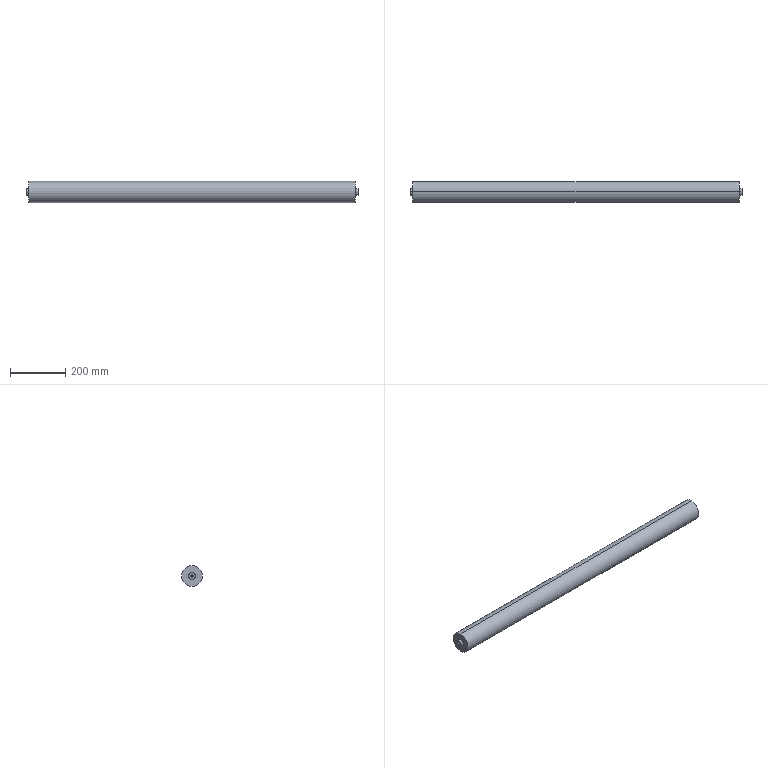Part | STEP file | φ76-1200 | 1 solid | 18 faces | box 1200 x 76 x 76 mm | volume 5359963 mm3 | cylinder 10 | cone 4 | plane 4 | commonest cylinder face diameters 8.5 x4 25 x4 76 x2
STEP:
#1=CARTESIAN_POINT('',(0.,0.,0.));
#2=DIRECTION('',(0.,0.,1.));
#3=DIRECTION('',(1.,0.,0.));
#4=AXIS2_PLACEMENT_3D('',#1,#2,#3);
#5=CARTESIAN_POINT('',(1175.5,0.,-4.25));
#6=VERTEX_POINT('',#5);
#7=CARTESIAN_POINT('',(1200.,0.,-4.25));
#8=VERTEX_POINT('',#7);
#9=CARTESIAN_POINT('',(1200.,0.,-4.25));
#10=DIRECTION('',(1.,0.,0.));
#11=VECTOR('',#10,1.);
#12=LINE('',#9,#11);
#13=CARTESIAN_POINT('',(1200.,0.,0.));
#14=DIRECTION('',(1.,0.,0.));
#15=DIRECTION('',(0.,0.,-1.));
#16=AXIS2_PLACEMENT_3D('',#13,#14,#15);
#17=CYLINDRICAL_SURFACE('',#16,4.25);
#18=CARTESIAN_POINT('',(6.283,0.));
#19=DIRECTION('',(0.,1.));
#20=VECTOR('',#19,1.);
#21=LINE('',#18,#20);
#22=(GEOMETRIC_REPRESENTATION_CONTEXT(2)PARAMETRIC_REPRESENTATION_CONTEXT()REPRESENTATION_CONTEXT('',''));
#23=DEFINITIONAL_REPRESENTATION('',(#21),#22);
#24=PCURVE('',#17,#23);
#25=CARTESIAN_POINT('',(1200.,0.,0.));
#26=DIRECTION('',(1.,0.,0.));
#27=DIRECTION('',(0.,0.,-1.));
#28=AXIS2_PLACEMENT_3D('',#25,#26,#27);
#29=CYLINDRICAL_SURFACE('',#28,4.25);
#30=CARTESIAN_POINT('',(0.,0.));
#31=DIRECTION('',(0.,1.));
#32=VECTOR('',#31,1.);
#33=LINE('',#30,#32);
#34=(GEOMETRIC_REPRESENTATION_CONTEXT(2)PARAMETRIC_REPRESENTATION_CONTEXT()REPRESENTATION_CONTEXT('',''));
#35=DEFINITIONAL_REPRESENTATION('',(#33),#34);
#36=PCURVE('',#29,#35);
#37=SURFACE_CURVE('',#12,(#24,#36),.PCURVE_S1.);
#38=EDGE_CURVE('',#6,#8,#37,.T.);
#39=ORIENTED_EDGE('',*,*,#38,.T.);
#40=CARTESIAN_POINT('',(1200.,0.,4.25));
#41=VERTEX_POINT('',#40);
#42=CARTESIAN_POINT('',(1200.,0.,0.));
#43=DIRECTION('',(1.,0.,0.));
#44=DIRECTION('',(0.,0.,-1.));
#45=AXIS2_PLACEMENT_3D('',#42,#43,#44);
#46=CIRCLE('',#45,4.25);
#47=CARTESIAN_POINT('',(0.,0.));
#48=DIRECTION('',(1.,0.));
#49=VECTOR('',#48,1.);
#50=LINE('',#47,#49);
#51=(GEOMETRIC_REPRESENTATION_CONTEXT(2)PARAMETRIC_REPRESENTATION_CONTEXT()REPRESENTATION_CONTEXT('',''));
#52=DEFINITIONAL_REPRESENTATION('',(#50),#51);
#53=PCURVE('',#17,#52);
#54=CARTESIAN_POINT('',(1200.,0.,0.));
#55=DIRECTION('',(-1.,0.,0.));
#56=DIRECTION('',(0.,0.,1.));
#57=AXIS2_PLACEMENT_3D('',#54,#55,#56);
#58=PLANE('',#57);
#59=CARTESIAN_POINT('',(-4.25,0.));
#60=CARTESIAN_POINT('',(-4.25,7.361));
#61=CARTESIAN_POINT('',(2.125,3.681));
#62=CARTESIAN_POINT('',(8.5,0.));
#63=CARTESIAN_POINT('',(2.125,-3.681));
#64=CARTESIAN_POINT('',(-4.25,-7.361));
#65=CARTESIAN_POINT('',(-4.25,0.));
#66=(BOUNDED_CURVE()B_SPLINE_CURVE(2,(#59,#60,#61,#62,#63,#64,#65),.UNSPECIFIED.,.T.,.F.)B_SPLINE_CURVE_WITH_KNOTS((1,2,2,2,2,1),(-2.094,0.,2.094,4.189,6.283,8.378),.UNSPECIFIED.)CURVE()GEOMETRIC_REPRESENTATION_ITEM()RATIONAL_B_SPLINE_CURVE((1.,0.5,1.,0.5,1.,0.5,1.))REPRESENTATION_ITEM(''));
#67=(GEOMETRIC_REPRESENTATION_CONTEXT(2)PARAMETRIC_REPRESENTATION_CONTEXT()REPRESENTATION_CONTEXT('',''));
#68=DEFINITIONAL_REPRESENTATION('',(#66),#67);
#69=PCURVE('',#58,#68);
#70=SURFACE_CURVE('',#46,(#53,#69),.PCURVE_S1.);
#71=EDGE_CURVE('',#41,#8,#70,.T.);
#72=ORIENTED_EDGE('',*,*,#71,.F.);
#73=CARTESIAN_POINT('',(1175.5,0.,4.25));
#74=VERTEX_POINT('',#73);
#75=CARTESIAN_POINT('',(1200.,0.,4.25));
#76=DIRECTION('',(1.,0.,0.));
#77=VECTOR('',#76,1.);
#78=LINE('',#75,#77);
#79=CARTESIAN_POINT('',(3.142,0.));
#80=DIRECTION('',(0.,1.));
#81=VECTOR('',#80,1.);
#82=LINE('',#79,#81);
#83=(GEOMETRIC_REPRESENTATION_CONTEXT(2)PARAMETRIC_REPRESENTATION_CONTEXT()REPRESENTATION_CONTEXT('',''));
#84=DEFINITIONAL_REPRESENTATION('',(#82),#83);
#85=PCURVE('',#17,#84);
#86=CARTESIAN_POINT('',(3.142,0.));
#87=DIRECTION('',(0.,1.));
#88=VECTOR('',#87,1.);
#89=LINE('',#86,#88);
#90=(GEOMETRIC_REPRESENTATION_CONTEXT(2)PARAMETRIC_REPRESENTATION_CONTEXT()REPRESENTATION_CONTEXT('',''));
#91=DEFINITIONAL_REPRESENTATION('',(#89),#90);
#92=PCURVE('',#29,#91);
#93=SURFACE_CURVE('',#78,(#85,#92),.PCURVE_S1.);
#94=EDGE_CURVE('',#74,#41,#93,.T.);
#95=ORIENTED_EDGE('',*,*,#94,.F.);
#96=CARTESIAN_POINT('',(1175.5,0.,0.));
#97=DIRECTION('',(1.,0.,0.));
#98=DIRECTION('',(0.,0.,-1.));
#99=AXIS2_PLACEMENT_3D('',#96,#97,#98);
#100=CIRCLE('',#99,4.25);
#101=CARTESIAN_POINT('',(0.,-24.5));
#102=DIRECTION('',(1.,0.));
#103=VECTOR('',#102,1.);
#104=LINE('',#101,#103);
#105=(GEOMETRIC_REPRESENTATION_CONTEXT(2)PARAMETRIC_REPRESENTATION_CONTEXT()REPRESENTATION_CONTEXT('',''));
#106=DEFINITIONAL_REPRESENTATION('',(#104),#105);
#107=PCURVE('',#17,#106);
#108=CARTESIAN_POINT('',(1175.5,0.,0.));
#109=DIRECTION('',(1.,0.,0.));
#110=DIRECTION('',(0.,0.,-1.));
#111=AXIS2_PLACEMENT_3D('',#108,#109,#110);
#112=CONICAL_SURFACE('',#111,4.25,1.03);
#113=CARTESIAN_POINT('',(0.,0.));
#114=DIRECTION('',(1.,0.));
#115=VECTOR('',#114,1.);
#116=LINE('',#113,#115);
#117=(GEOMETRIC_REPRESENTATION_CONTEXT(2)PARAMETRIC_REPRESENTATION_CONTEXT()REPRESENTATION_CONTEXT('',''));
#118=DEFINITIONAL_REPRESENTATION('',(#116),#117);
#119=PCURVE('',#112,#118);
#120=SURFACE_CURVE('',#100,(#107,#119),.PCURVE_S1.);
#121=EDGE_CURVE('',#74,#6,#120,.T.);
#122=ORIENTED_EDGE('',*,*,#121,.T.);
#123=EDGE_LOOP('',(#39,#72,#95,#122));
#124=FACE_BOUND('',#123,.F.);
#125=ADVANCED_FACE('',(#124),#17,.F.);
#126=ORIENTED_EDGE('',*,*,#121,.F.);
#127=CARTESIAN_POINT('',(1172.946,0.,0.));
#128=VERTEX_POINT('',#127);
#129=CARTESIAN_POINT('',(1175.5,0.,4.25));
#130=DIRECTION('',(0.515,0.,0.8572));
#131=VECTOR('',#130,1.);
#132=LINE('',#129,#131);
#133=CARTESIAN_POINT('',(3.142,0.));
#134=DIRECTION('',(0.,1.));
#135=VECTOR('',#134,1.);
#136=LINE('',#133,#135);
#137=(GEOMETRIC_REPRESENTATION_CONTEXT(2)PARAMETRIC_REPRESENTATION_CONTEXT()REPRESENTATION_CONTEXT('',''));
#138=DEFINITIONAL_REPRESENTATION('',(#136),#137);
#139=PCURVE('',#112,#138);
#140=CARTESIAN_POINT('',(1175.5,0.,0.));
#141=DIRECTION('',(1.,0.,0.));
#142=DIRECTION('',(0.,0.,-1.));
#143=AXIS2_PLACEMENT_3D('',#140,#141,#142);
#144=CONICAL_SURFACE('',#143,4.25,1.03);
#145=CARTESIAN_POINT('',(3.142,0.));
#146=DIRECTION('',(0.,1.));
#147=VECTOR('',#146,1.);
#148=LINE('',#145,#147);
#149=(GEOMETRIC_REPRESENTATION_CONTEXT(2)PARAMETRIC_REPRESENTATION_CONTEXT()REPRESENTATION_CONTEXT('',''));
#150=DEFINITIONAL_REPRESENTATION('',(#148),#149);
#151=PCURVE('',#144,#150);
#152=SURFACE_CURVE('',#132,(#139,#151),.PCURVE_S1.);
#153=EDGE_CURVE('',#128,#74,#152,.T.);
#154=ORIENTED_EDGE('',*,*,#153,.F.);
#155=CARTESIAN_POINT('',(1175.5,0.,-4.25));
#156=DIRECTION('',(0.515,0.,-0.8572));
#157=VECTOR('',#156,1.);
#158=LINE('',#155,#157);
#159=CARTESIAN_POINT('',(6.283,0.));
#160=DIRECTION('',(0.,1.));
#161=VECTOR('',#160,1.);
#162=LINE('',#159,#161);
#163=(GEOMETRIC_REPRESENTATION_CONTEXT(2)PARAMETRIC_REPRESENTATION_CONTEXT()REPRESENTATION_CONTEXT('',''));
#164=DEFINITIONAL_REPRESENTATION('',(#162),#163);
#165=PCURVE('',#112,#164);
#166=CARTESIAN_POINT('',(0.,0.));
#167=DIRECTION('',(0.,1.));
#168=VECTOR('',#167,1.);
#169=LINE('',#166,#168);
#170=(GEOMETRIC_REPRESENTATION_CONTEXT(2)PARAMETRIC_REPRESENTATION_CONTEXT()REPRESENTATION_CONTEXT('',''));
#171=DEFINITIONAL_REPRESENTATION('',(#169),#170);
#172=PCURVE('',#144,#171);
#173=SURFACE_CURVE('',#158,(#165,#172),.PCURVE_S1.);
#174=EDGE_CURVE('',#128,#6,#173,.T.);
#175=ORIENTED_EDGE('',*,*,#174,.T.);
#176=EDGE_LOOP('',(#126,#154,#175));
#177=FACE_BOUND('',#176,.F.);
#178=ADVANCED_FACE('',(#177),#112,.F.);
#179=CARTESIAN_POINT('',(24.5,0.,4.25));
#180=VERTEX_POINT('',#179);
#181=CARTESIAN_POINT('',(0.,0.,4.25));
#182=VERTEX_POINT('',#181);
#183=CARTESIAN_POINT('',(0.,0.,4.25));
#184=DIRECTION('',(-1.,0.,0.));
#185=VECTOR('',#184,1.);
#186=LINE('',#183,#185);
#187=CARTESIAN_POINT('',(0.,0.,0.));
#188=DIRECTION('',(-1.,0.,0.));
#189=DIRECTION('',(0.,0.,1.));
#190=AXIS2_PLACEMENT_3D('',#187,#188,#189);
#191=CYLINDRICAL_SURFACE('',#190,4.25);
#192=CARTESIAN_POINT('',(6.283,0.));
#193=DIRECTION('',(0.,1.));
#194=VECTOR('',#193,1.);
#195=LINE('',#192,#194);
#196=(GEOMETRIC_REPRESENTATION_CONTEXT(2)PARAMETRIC_REPRESENTATION_CONTEXT()REPRESENTATION_CONTEXT('',''));
#197=DEFINITIONAL_REPRESENTATION('',(#195),#196);
#198=PCURVE('',#191,#197);
#199=CARTESIAN_POINT('',(0.,0.,0.));
#200=DIRECTION('',(-1.,0.,0.));
#201=DIRECTION('',(0.,0.,1.));
#202=AXIS2_PLACEMENT_3D('',#199,#200,#201);
#203=CYLINDRICAL_SURFACE('',#202,4.25);
#204=CARTESIAN_POINT('',(0.,0.));
#205=DIRECTION('',(0.,1.));
#206=VECTOR('',#205,1.);
#207=LINE('',#204,#206);
#208=(GEOMETRIC_REPRESENTATION_CONTEXT(2)PARAMETRIC_REPRESENTATION_CONTEXT()REPRESENTATION_CONTEXT('',''));
#209=DEFINITIONAL_REPRESENTATION('',(#207),#208);
#210=PCURVE('',#203,#209);
#211=SURFACE_CURVE('',#186,(#198,#210),.PCURVE_S1.);
#212=EDGE_CURVE('',#180,#182,#211,.T.);
#213=ORIENTED_EDGE('',*,*,#212,.T.);
#214=CARTESIAN_POINT('',(0.,0.,-4.25));
#215=VERTEX_POINT('',#214);
#216=CARTESIAN_POINT('',(0.,0.,0.));
#217=DIRECTION('',(-1.,0.,0.));
#218=DIRECTION('',(0.,0.,1.));
#219=AXIS2_PLACEMENT_3D('',#216,#217,#218);
#220=CIRCLE('',#219,4.25);
#221=CARTESIAN_POINT('',(0.,0.));
#222=DIRECTION('',(1.,0.));
#223=VECTOR('',#222,1.);
#224=LINE('',#221,#223);
#225=(GEOMETRIC_REPRESENTATION_CONTEXT(2)PARAMETRIC_REPRESENTATION_CONTEXT()REPRESENTATION_CONTEXT('',''));
#226=DEFINITIONAL_REPRESENTATION('',(#224),#225);
#227=PCURVE('',#191,#226);
#228=CARTESIAN_POINT('',(0.,0.,0.));
#229=DIRECTION('',(1.,0.,0.));
#230=DIRECTION('',(0.,0.,-1.));
#231=AXIS2_PLACEMENT_3D('',#228,#229,#230);
#232=PLANE('',#231);
#233=CARTESIAN_POINT('',(-4.25,0.));
#234=CARTESIAN_POINT('',(-4.25,7.361));
#235=CARTESIAN_POINT('',(2.125,3.681));
#236=CARTESIAN_POINT('',(8.5,0.));
#237=CARTESIAN_POINT('',(2.125,-3.681));
#238=CARTESIAN_POINT('',(-4.25,-7.361));
#239=CARTESIAN_POINT('',(-4.25,0.));
#240=(BOUNDED_CURVE()B_SPLINE_CURVE(2,(#233,#234,#235,#236,#237,#238,#239),.UNSPECIFIED.,.T.,.F.)B_SPLINE_CURVE_WITH_KNOTS((1,2,2,2,2,1),(-2.094,0.,2.094,4.189,6.283,8.378),.UNSPECIFIED.)CURVE()GEOMETRIC_REPRESENTATION_ITEM()RATIONAL_B_SPLINE_CURVE((1.,0.5,1.,0.5,1.,0.5,1.))REPRESENTATION_ITEM(''));
#241=(GEOMETRIC_REPRESENTATION_CONTEXT(2)PARAMETRIC_REPRESENTATION_CONTEXT()REPRESENTATION_CONTEXT('',''));
#242=DEFINITIONAL_REPRESENTATION('',(#240),#241);
#243=PCURVE('',#232,#242);
#244=SURFACE_CURVE('',#220,(#227,#243),.PCURVE_S1.);
#245=EDGE_CURVE('',#215,#182,#244,.T.);
#246=ORIENTED_EDGE('',*,*,#245,.F.);
#247=CARTESIAN_POINT('',(24.5,0.,-4.25));
#248=VERTEX_POINT('',#247);
#249=CARTESIAN_POINT('',(0.,0.,-4.25));
#250=DIRECTION('',(-1.,0.,0.));
#251=VECTOR('',#250,1.);
#252=LINE('',#249,#251);
#253=CARTESIAN_POINT('',(3.142,0.));
#254=DIRECTION('',(0.,1.));
#255=VECTOR('',#254,1.);
#256=LINE('',#253,#255);
#257=(GEOMETRIC_REPRESENTATION_CONTEXT(2)PARAMETRIC_REPRESENTATION_CONTEXT()REPRESENTATION_CONTEXT('',''));
#258=DEFINITIONAL_REPRESENTATION('',(#256),#257);
#259=PCURVE('',#191,#258);
#260=CARTESIAN_POINT('',(3.142,0.));
#261=DIRECTION('',(0.,1.));
#262=VECTOR('',#261,1.);
#263=LINE('',#260,#262);
#264=(GEOMETRIC_REPRESENTATION_CONTEXT(2)PARAMETRIC_REPRESENTATION_CONTEXT()REPRESENTATION_CONTEXT('',''));
#265=DEFINITIONAL_REPRESENTATION('',(#263),#264);
#266=PCURVE('',#203,#265);
#267=SURFACE_CURVE('',#252,(#259,#266),.PCURVE_S1.);
#268=EDGE_CURVE('',#248,#215,#267,.T.);
#269=ORIENTED_EDGE('',*,*,#268,.F.);
#270=CARTESIAN_POINT('',(24.5,0.,0.));
#271=DIRECTION('',(-1.,0.,0.));
#272=DIRECTION('',(0.,0.,1.));
#273=AXIS2_PLACEMENT_3D('',#270,#271,#272);
#274=CIRCLE('',#273,4.25);
#275=CARTESIAN_POINT('',(0.,-24.5));
#276=DIRECTION('',(1.,0.));
#277=VECTOR('',#276,1.);
#278=LINE('',#275,#277);
#279=(GEOMETRIC_REPRESENTATION_CONTEXT(2)PARAMETRIC_REPRESENTATION_CONTEXT()REPRESENTATION_CONTEXT('',''));
#280=DEFINITIONAL_REPRESENTATION('',(#278),#279);
#281=PCURVE('',#191,#280);
#282=CARTESIAN_POINT('',(24.5,0.,0.));
#283=DIRECTION('',(-1.,0.,0.));
#284=DIRECTION('',(0.,0.,1.));
#285=AXIS2_PLACEMENT_3D('',#282,#283,#284);
#286=CONICAL_SURFACE('',#285,4.25,1.03);
#287=CARTESIAN_POINT('',(0.,0.));
#288=DIRECTION('',(1.,0.));
#289=VECTOR('',#288,1.);
#290=LINE('',#287,#289);
#291=(GEOMETRIC_REPRESENTATION_CONTEXT(2)PARAMETRIC_REPRESENTATION_CONTEXT()REPRESENTATION_CONTEXT('',''));
#292=DEFINITIONAL_REPRESENTATION('',(#290),#291);
#293=PCURVE('',#286,#292);
#294=SURFACE_CURVE('',#274,(#281,#293),.PCURVE_S1.);
#295=EDGE_CURVE('',#248,#180,#294,.T.);
#296=ORIENTED_EDGE('',*,*,#295,.T.);
#297=EDGE_LOOP('',(#213,#246,#269,#296));
#298=FACE_BOUND('',#297,.F.);
#299=ADVANCED_FACE('',(#298),#191,.F.);
#300=ORIENTED_EDGE('',*,*,#295,.F.);
#301=CARTESIAN_POINT('',(27.054,0.,0.));
#302=VERTEX_POINT('',#301);
#303=CARTESIAN_POINT('',(24.5,0.,-4.25));
#304=DIRECTION('',(-0.515,0.,-0.8572));
#305=VECTOR('',#304,1.);
#306=LINE('',#303,#305);
#307=CARTESIAN_POINT('',(3.142,0.));
#308=DIRECTION('',(0.,1.));
#309=VECTOR('',#308,1.);
#310=LINE('',#307,#309);
#311=(GEOMETRIC_REPRESENTATION_CONTEXT(2)PARAMETRIC_REPRESENTATION_CONTEXT()REPRESENTATION_CONTEXT('',''));
#312=DEFINITIONAL_REPRESENTATION('',(#310),#311);
#313=PCURVE('',#286,#312);
#314=CARTESIAN_POINT('',(24.5,0.,0.));
#315=DIRECTION('',(-1.,0.,0.));
#316=DIRECTION('',(0.,0.,1.));
#317=AXIS2_PLACEMENT_3D('',#314,#315,#316);
#318=CONICAL_SURFACE('',#317,4.25,1.03);
#319=CARTESIAN_POINT('',(3.142,0.));
#320=DIRECTION('',(0.,1.));
#321=VECTOR('',#320,1.);
#322=LINE('',#319,#321);
#323=(GEOMETRIC_REPRESENTATION_CONTEXT(2)PARAMETRIC_REPRESENTATION_CONTEXT()REPRESENTATION_CONTEXT('',''));
#324=DEFINITIONAL_REPRESENTATION('',(#322),#323);
#325=PCURVE('',#318,#324);
#326=SURFACE_CURVE('',#306,(#313,#325),.PCURVE_S1.);
#327=EDGE_CURVE('',#302,#248,#326,.T.);
#328=ORIENTED_EDGE('',*,*,#327,.F.);
#329=CARTESIAN_POINT('',(24.5,0.,4.25));
#330=DIRECTION('',(-0.515,0.,0.8572));
#331=VECTOR('',#330,1.);
#332=LINE('',#329,#331);
#333=CARTESIAN_POINT('',(6.283,0.));
#334=DIRECTION('',(0.,1.));
#335=VECTOR('',#334,1.);
#336=LINE('',#333,#335);
#337=(GEOMETRIC_REPRESENTATION_CONTEXT(2)PARAMETRIC_REPRESENTATION_CONTEXT()REPRESENTATION_CONTEXT('',''));
#338=DEFINITIONAL_REPRESENTATION('',(#336),#337);
#339=PCURVE('',#286,#338);
#340=CARTESIAN_POINT('',(0.,0.));
#341=DIRECTION('',(0.,1.));
#342=VECTOR('',#341,1.);
#343=LINE('',#340,#342);
#344=(GEOMETRIC_REPRESENTATION_CONTEXT(2)PARAMETRIC_REPRESENTATION_CONTEXT()REPRESENTATION_CONTEXT('',''));
#345=DEFINITIONAL_REPRESENTATION('',(#343),#344);
#346=PCURVE('',#318,#345);
#347=SURFACE_CURVE('',#332,(#339,#346),.PCURVE_S1.);
#348=EDGE_CURVE('',#302,#180,#347,.T.);
#349=ORIENTED_EDGE('',*,*,#348,.T.);
#350=EDGE_LOOP('',(#300,#328,#349));
#351=FACE_BOUND('',#350,.F.);
#352=ADVANCED_FACE('',(#351),#286,.F.);
#353=CARTESIAN_POINT('',(10.,0.,12.5));
#354=VERTEX_POINT('',#353);
#355=CARTESIAN_POINT('',(10.,0.,-12.5));
#356=VERTEX_POINT('',#355);
#357=CARTESIAN_POINT('',(10.,0.,0.));
#358=DIRECTION('',(-1.,0.,0.));
#359=DIRECTION('',(0.,0.,1.));
#360=AXIS2_PLACEMENT_3D('',#357,#358,#359);
#361=CIRCLE('',#360,12.5);
#362=CARTESIAN_POINT('',(0.,0.,0.));
#363=DIRECTION('',(-1.,0.,0.));
#364=DIRECTION('',(0.,0.,1.));
#365=AXIS2_PLACEMENT_3D('',#362,#363,#364);
#366=CYLINDRICAL_SURFACE('',#365,12.5);
#367=CARTESIAN_POINT('',(0.,-10.));
#368=DIRECTION('',(1.,0.));
#369=VECTOR('',#368,1.);
#370=LINE('',#367,#369);
#371=(GEOMETRIC_REPRESENTATION_CONTEXT(2)PARAMETRIC_REPRESENTATION_CONTEXT()REPRESENTATION_CONTEXT('',''));
#372=DEFINITIONAL_REPRESENTATION('',(#370),#371);
#373=PCURVE('',#366,#372);
#374=CARTESIAN_POINT('',(10.,38.,0.));
#375=DIRECTION('',(1.,0.,0.));
#376=DIRECTION('',(0.,0.,-1.));
#377=AXIS2_PLACEMENT_3D('',#374,#375,#376);
#378=PLANE('',#377);
#379=CARTESIAN_POINT('',(-12.5,-38.));
#380=CARTESIAN_POINT('',(-12.5,-16.349));
#381=CARTESIAN_POINT('',(6.25,-27.175));
#382=CARTESIAN_POINT('',(25.,-38.));
#383=CARTESIAN_POINT('',(6.25,-48.825));
#384=CARTESIAN_POINT('',(-12.5,-59.651));
#385=CARTESIAN_POINT('',(-12.5,-38.));
#386=(BOUNDED_CURVE()B_SPLINE_CURVE(2,(#379,#380,#381,#382,#383,#384,#385),.UNSPECIFIED.,.T.,.F.)B_SPLINE_CURVE_WITH_KNOTS((1,2,2,2,2,1),(-2.094,0.,2.094,4.189,6.283,8.378),.UNSPECIFIED.)CURVE()GEOMETRIC_REPRESENTATION_ITEM()RATIONAL_B_SPLINE_CURVE((1.,0.5,1.,0.5,1.,0.5,1.))REPRESENTATION_ITEM(''));
#387=(GEOMETRIC_REPRESENTATION_CONTEXT(2)PARAMETRIC_REPRESENTATION_CONTEXT()REPRESENTATION_CONTEXT('',''));
#388=DEFINITIONAL_REPRESENTATION('',(#386),#387);
#389=PCURVE('',#378,#388);
#390=SURFACE_CURVE('',#361,(#373,#389),.PCURVE_S1.);
#391=EDGE_CURVE('',#354,#356,#390,.T.);
#392=ORIENTED_EDGE('',*,*,#391,.T.);
#393=CARTESIAN_POINT('',(0.,0.,-12.5));
#394=VERTEX_POINT('',#393);
#395=CARTESIAN_POINT('',(0.,0.,-12.5));
#396=DIRECTION('',(-1.,0.,0.));
#397=VECTOR('',#396,1.);
#398=LINE('',#395,#397);
#399=CARTESIAN_POINT('',(3.142,0.));
#400=DIRECTION('',(0.,1.));
#401=VECTOR('',#400,1.);
#402=LINE('',#399,#401);
#403=(GEOMETRIC_REPRESENTATION_CONTEXT(2)PARAMETRIC_REPRESENTATION_CONTEXT()REPRESENTATION_CONTEXT('',''));
#404=DEFINITIONAL_REPRESENTATION('',(#402),#403);
#405=PCURVE('',#366,#404);
#406=CARTESIAN_POINT('',(0.,0.,0.));
#407=DIRECTION('',(-1.,0.,0.));
#408=DIRECTION('',(0.,0.,1.));
#409=AXIS2_PLACEMENT_3D('',#406,#407,#408);
#410=CYLINDRICAL_SURFACE('',#409,12.5);
#411=CARTESIAN_POINT('',(3.142,0.));
#412=DIRECTION('',(0.,1.));
#413=VECTOR('',#412,1.);
#414=LINE('',#411,#413);
#415=(GEOMETRIC_REPRESENTATION_CONTEXT(2)PARAMETRIC_REPRESENTATION_CONTEXT()REPRESENTATION_CONTEXT('',''));
#416=DEFINITIONAL_REPRESENTATION('',(#414),#415);
#417=PCURVE('',#410,#416);
#418=SURFACE_CURVE('',#398,(#405,#417),.PCURVE_S1.);
#419=EDGE_CURVE('',#356,#394,#418,.T.);
#420=ORIENTED_EDGE('',*,*,#419,.T.);
#421=CARTESIAN_POINT('',(0.,0.,12.5));
#422=VERTEX_POINT('',#421);
#423=CARTESIAN_POINT('',(0.,0.,0.));
#424=DIRECTION('',(-1.,0.,0.));
#425=DIRECTION('',(0.,0.,1.));
#426=AXIS2_PLACEMENT_3D('',#423,#424,#425);
#427=CIRCLE('',#426,12.5);
#428=CARTESIAN_POINT('',(0.,0.));
#429=DIRECTION('',(1.,0.));
#430=VECTOR('',#429,1.);
#431=LINE('',#428,#430);
#432=(GEOMETRIC_REPRESENTATION_CONTEXT(2)PARAMETRIC_REPRESENTATION_CONTEXT()REPRESENTATION_CONTEXT('',''));
#433=DEFINITIONAL_REPRESENTATION('',(#431),#432);
#434=PCURVE('',#366,#433);
#435=CARTESIAN_POINT('',(-12.5,0.));
#436=CARTESIAN_POINT('',(-12.5,21.651));
#437=CARTESIAN_POINT('',(6.25,10.825));
#438=CARTESIAN_POINT('',(25.,0.));
#439=CARTESIAN_POINT('',(6.25,-10.825));
#440=CARTESIAN_POINT('',(-12.5,-21.651));
#441=CARTESIAN_POINT('',(-12.5,0.));
#442=(BOUNDED_CURVE()B_SPLINE_CURVE(2,(#435,#436,#437,#438,#439,#440,#441),.UNSPECIFIED.,.T.,.F.)B_SPLINE_CURVE_WITH_KNOTS((1,2,2,2,2,1),(-2.094,0.,2.094,4.189,6.283,8.378),.UNSPECIFIED.)CURVE()GEOMETRIC_REPRESENTATION_ITEM()RATIONAL_B_SPLINE_CURVE((1.,0.5,1.,0.5,1.,0.5,1.))REPRESENTATION_ITEM(''));
#443=(GEOMETRIC_REPRESENTATION_CONTEXT(2)PARAMETRIC_REPRESENTATION_CONTEXT()REPRESENTATION_CONTEXT('',''));
#444=DEFINITIONAL_REPRESENTATION('',(#442),#443);
#445=PCURVE('',#232,#444);
#446=SURFACE_CURVE('',#427,(#434,#445),.PCURVE_S1.);
#447=EDGE_CURVE('',#422,#394,#446,.T.);
#448=ORIENTED_EDGE('',*,*,#447,.F.);
#449=CARTESIAN_POINT('',(0.,0.,12.5));
#450=DIRECTION('',(-1.,0.,0.));
#451=VECTOR('',#450,1.);
#452=LINE('',#449,#451);
#453=CARTESIAN_POINT('',(0.,0.));
#454=DIRECTION('',(0.,1.));
#455=VECTOR('',#454,1.);
#456=LINE('',#453,#455);
#457=(GEOMETRIC_REPRESENTATION_CONTEXT(2)PARAMETRIC_REPRESENTATION_CONTEXT()REPRESENTATION_CONTEXT('',''));
#458=DEFINITIONAL_REPRESENTATION('',(#456),#457);
#459=PCURVE('',#366,#458);
#460=CARTESIAN_POINT('',(6.283,0.));
#461=DIRECTION('',(0.,1.));
#462=VECTOR('',#461,1.);
#463=LINE('',#460,#462);
#464=(GEOMETRIC_REPRESENTATION_CONTEXT(2)PARAMETRIC_REPRESENTATION_CONTEXT()REPRESENTATION_CONTEXT('',''));
#465=DEFINITIONAL_REPRESENTATION('',(#463),#464);
#466=PCURVE('',#410,#465);
#467=SURFACE_CURVE('',#452,(#459,#466),.PCURVE_S1.);
#468=EDGE_CURVE('',#354,#422,#467,.T.);
#469=ORIENTED_EDGE('',*,*,#468,.F.);
#470=EDGE_LOOP('',(#392,#420,#448,#469));
#471=FACE_BOUND('',#470,.T.);
#472=ADVANCED_FACE('',(#471),#366,.T.);
#473=CARTESIAN_POINT('',(1190.,0.,38.));
#474=VERTEX_POINT('',#473);
#475=CARTESIAN_POINT('',(1190.,0.,-38.));
#476=VERTEX_POINT('',#475);
#477=CARTESIAN_POINT('',(1190.,0.,0.));
#478=DIRECTION('',(-1.,0.,0.));
#479=DIRECTION('',(0.,0.,1.));
#480=AXIS2_PLACEMENT_3D('',#477,#478,#479);
#481=CIRCLE('',#480,38.);
#482=CARTESIAN_POINT('',(0.,0.,0.));
#483=DIRECTION('',(-1.,0.,0.));
#484=DIRECTION('',(0.,0.,1.));
#485=AXIS2_PLACEMENT_3D('',#482,#483,#484);
#486=CYLINDRICAL_SURFACE('',#485,38.);
#487=CARTESIAN_POINT('',(0.,-1190.));
#488=DIRECTION('',(1.,0.));
#489=VECTOR('',#488,1.);
#490=LINE('',#487,#489);
#491=(GEOMETRIC_REPRESENTATION_CONTEXT(2)PARAMETRIC_REPRESENTATION_CONTEXT()REPRESENTATION_CONTEXT('',''));
#492=DEFINITIONAL_REPRESENTATION('',(#490),#491);
#493=PCURVE('',#486,#492);
#494=CARTESIAN_POINT('',(1190.,12.5,0.));
#495=DIRECTION('',(-1.,0.,0.));
#496=DIRECTION('',(0.,0.,1.));
#497=AXIS2_PLACEMENT_3D('',#494,#495,#496);
#498=PLANE('',#497);
#499=CARTESIAN_POINT('',(0.,-12.5));
#500=DIRECTION('',(1.,0.));
#501=AXIS2_PLACEMENT_2D('',#499,#500);
#502=CIRCLE('',#501,38.);
#503=(GEOMETRIC_REPRESENTATION_CONTEXT(2)PARAMETRIC_REPRESENTATION_CONTEXT()REPRESENTATION_CONTEXT('',''));
#504=DEFINITIONAL_REPRESENTATION('',(#502),#503);
#505=PCURVE('',#498,#504);
#506=SURFACE_CURVE('',#481,(#493,#505),.PCURVE_S1.);
#507=EDGE_CURVE('',#474,#476,#506,.T.);
#508=ORIENTED_EDGE('',*,*,#507,.T.);
#509=CARTESIAN_POINT('',(10.,0.,-38.));
#510=VERTEX_POINT('',#509);
#511=CARTESIAN_POINT('',(0.,0.,-38.));
#512=DIRECTION('',(-1.,0.,0.));
#513=VECTOR('',#512,1.);
#514=LINE('',#511,#513);
#515=CARTESIAN_POINT('',(3.142,0.));
#516=DIRECTION('',(0.,1.));
#517=VECTOR('',#516,1.);
#518=LINE('',#515,#517);
#519=(GEOMETRIC_REPRESENTATION_CONTEXT(2)PARAMETRIC_REPRESENTATION_CONTEXT()REPRESENTATION_CONTEXT('',''));
#520=DEFINITIONAL_REPRESENTATION('',(#518),#519);
#521=PCURVE('',#486,#520);
#522=CARTESIAN_POINT('',(0.,0.,0.));
#523=DIRECTION('',(-1.,0.,0.));
#524=DIRECTION('',(0.,0.,1.));
#525=AXIS2_PLACEMENT_3D('',#522,#523,#524);
#526=CYLINDRICAL_SURFACE('',#525,38.);
#527=CARTESIAN_POINT('',(3.142,0.));
#528=DIRECTION('',(0.,1.));
#529=VECTOR('',#528,1.);
#530=LINE('',#527,#529);
#531=(GEOMETRIC_REPRESENTATION_CONTEXT(2)PARAMETRIC_REPRESENTATION_CONTEXT()REPRESENTATION_CONTEXT('',''));
#532=DEFINITIONAL_REPRESENTATION('',(#530),#531);
#533=PCURVE('',#526,#532);
#534=SURFACE_CURVE('',#514,(#521,#533),.PCURVE_S1.);
#535=EDGE_CURVE('',#476,#510,#534,.T.);
#536=ORIENTED_EDGE('',*,*,#535,.T.);
#537=CARTESIAN_POINT('',(10.,0.,38.));
#538=VERTEX_POINT('',#537);
#539=CARTESIAN_POINT('',(10.,0.,0.));
#540=DIRECTION('',(-1.,0.,0.));
#541=DIRECTION('',(0.,0.,1.));
#542=AXIS2_PLACEMENT_3D('',#539,#540,#541);
#543=CIRCLE('',#542,38.);
#544=CARTESIAN_POINT('',(0.,-10.));
#545=DIRECTION('',(1.,0.));
#546=VECTOR('',#545,1.);
#547=LINE('',#544,#546);
#548=(GEOMETRIC_REPRESENTATION_CONTEXT(2)PARAMETRIC_REPRESENTATION_CONTEXT()REPRESENTATION_CONTEXT('',''));
#549=DEFINITIONAL_REPRESENTATION('',(#547),#548);
#550=PCURVE('',#486,#549);
#551=CARTESIAN_POINT('',(-38.,-38.));
#552=CARTESIAN_POINT('',(-38.,27.818));
#553=CARTESIAN_POINT('',(19.,-5.091));
#554=CARTESIAN_POINT('',(76.,-38.));
#555=CARTESIAN_POINT('',(19.,-70.909));
#556=CARTESIAN_POINT('',(-38.,-103.818));
#557=CARTESIAN_POINT('',(-38.,-38.));
#558=(BOUNDED_CURVE()B_SPLINE_CURVE(2,(#551,#552,#553,#554,#555,#556,#557),.UNSPECIFIED.,.T.,.F.)B_SPLINE_CURVE_WITH_KNOTS((1,2,2,2,2,1),(-2.094,0.,2.094,4.189,6.283,8.378),.UNSPECIFIED.)CURVE()GEOMETRIC_REPRESENTATION_ITEM()RATIONAL_B_SPLINE_CURVE((1.,0.5,1.,0.5,1.,0.5,1.))REPRESENTATION_ITEM(''));
#559=(GEOMETRIC_REPRESENTATION_CONTEXT(2)PARAMETRIC_REPRESENTATION_CONTEXT()REPRESENTATION_CONTEXT('',''));
#560=DEFINITIONAL_REPRESENTATION('',(#558),#559);
#561=PCURVE('',#378,#560);
#562=SURFACE_CURVE('',#543,(#550,#561),.PCURVE_S1.);
#563=EDGE_CURVE('',#538,#510,#562,.T.);
#564=ORIENTED_EDGE('',*,*,#563,.F.);
#565=CARTESIAN_POINT('',(0.,0.,38.));
#566=DIRECTION('',(-1.,0.,0.));
#567=VECTOR('',#566,1.);
#568=LINE('',#565,#567);
#569=CARTESIAN_POINT('',(0.,0.));
#570=DIRECTION('',(0.,1.));
#571=VECTOR('',#570,1.);
#572=LINE('',#569,#571);
#573=(GEOMETRIC_REPRESENTATION_CONTEXT(2)PARAMETRIC_REPRESENTATION_CONTEXT()REPRESENTATION_CONTEXT('',''));
#574=DEFINITIONAL_REPRESENTATION('',(#572),#573);
#575=PCURVE('',#486,#574);
#576=CARTESIAN_POINT('',(6.283,0.));
#577=DIRECTION('',(0.,1.));
#578=VECTOR('',#577,1.);
#579=LINE('',#576,#578);
#580=(GEOMETRIC_REPRESENTATION_CONTEXT(2)PARAMETRIC_REPRESENTATION_CONTEXT()REPRESENTATION_CONTEXT('',''));
#581=DEFINITIONAL_REPRESENTATION('',(#579),#580);
#582=PCURVE('',#526,#581);
#583=SURFACE_CURVE('',#568,(#575,#582),.PCURVE_S1.);
#584=EDGE_CURVE('',#474,#538,#583,.T.);
#585=ORIENTED_EDGE('',*,*,#584,.F.);
#586=EDGE_LOOP('',(#508,#536,#564,#585));
#587=FACE_BOUND('',#586,.T.);
#588=ADVANCED_FACE('',(#587),#486,.T.);
#589=CARTESIAN_POINT('',(1200.,0.,12.5));
#590=VERTEX_POINT('',#589);
#591=CARTESIAN_POINT('',(1200.,0.,-12.5));
#592=VERTEX_POINT('',#591);
#593=CARTESIAN_POINT('',(1200.,0.,0.));
#594=DIRECTION('',(-1.,0.,0.));
#595=DIRECTION('',(0.,0.,1.));
#596=AXIS2_PLACEMENT_3D('',#593,#594,#595);
#597=CIRCLE('',#596,12.5);
#598=CARTESIAN_POINT('',(0.,0.,0.));
#599=DIRECTION('',(-1.,0.,0.));
#600=DIRECTION('',(0.,0.,1.));
#601=AXIS2_PLACEMENT_3D('',#598,#599,#600);
#602=CYLINDRICAL_SURFACE('',#601,12.5);
#603=CARTESIAN_POINT('',(0.,-1200.));
#604=DIRECTION('',(1.,0.));
#605=VECTOR('',#604,1.);
#606=LINE('',#603,#605);
#607=(GEOMETRIC_REPRESENTATION_CONTEXT(2)PARAMETRIC_REPRESENTATION_CONTEXT()REPRESENTATION_CONTEXT('',''));
#608=DEFINITIONAL_REPRESENTATION('',(#606),#607);
#609=PCURVE('',#602,#608);
#610=CARTESIAN_POINT('',(0.,0.));
#611=DIRECTION('',(1.,0.));
#612=AXIS2_PLACEMENT_2D('',#610,#611);
#613=CIRCLE('',#612,12.5);
#614=(GEOMETRIC_REPRESENTATION_CONTEXT(2)PARAMETRIC_REPRESENTATION_CONTEXT()REPRESENTATION_CONTEXT('',''));
#615=DEFINITIONAL_REPRESENTATION('',(#613),#614);
#616=PCURVE('',#58,#615);
#617=SURFACE_CURVE('',#597,(#609,#616),.PCURVE_S1.);
#618=EDGE_CURVE('',#590,#592,#617,.T.);
#619=ORIENTED_EDGE('',*,*,#618,.T.);
#620=CARTESIAN_POINT('',(1190.,0.,-12.5));
#621=VERTEX_POINT('',#620);
#622=CARTESIAN_POINT('',(0.,0.,-12.5));
#623=DIRECTION('',(-1.,0.,0.));
#624=VECTOR('',#623,1.);
#625=LINE('',#622,#624);
#626=CARTESIAN_POINT('',(3.142,0.));
#627=DIRECTION('',(0.,1.));
#628=VECTOR('',#627,1.);
#629=LINE('',#626,#628);
#630=(GEOMETRIC_REPRESENTATION_CONTEXT(2)PARAMETRIC_REPRESENTATION_CONTEXT()REPRESENTATION_CONTEXT('',''));
#631=DEFINITIONAL_REPRESENTATION('',(#629),#630);
#632=PCURVE('',#602,#631);
#633=CARTESIAN_POINT('',(0.,0.,0.));
#634=DIRECTION('',(-1.,0.,0.));
#635=DIRECTION('',(0.,0.,1.));
#636=AXIS2_PLACEMENT_3D('',#633,#634,#635);
#637=CYLINDRICAL_SURFACE('',#636,12.5);
#638=CARTESIAN_POINT('',(3.142,0.));
#639=DIRECTION('',(0.,1.));
#640=VECTOR('',#639,1.);
#641=LINE('',#638,#640);
#642=(GEOMETRIC_REPRESENTATION_CONTEXT(2)PARAMETRIC_REPRESENTATION_CONTEXT()REPRESENTATION_CONTEXT('',''));
#643=DEFINITIONAL_REPRESENTATION('',(#641),#642);
#644=PCURVE('',#637,#643);
#645=SURFACE_CURVE('',#625,(#632,#644),.PCURVE_S1.);
#646=EDGE_CURVE('',#592,#621,#645,.T.);
#647=ORIENTED_EDGE('',*,*,#646,.T.);
#648=CARTESIAN_POINT('',(1190.,0.,12.5));
#649=VERTEX_POINT('',#648);
#650=CARTESIAN_POINT('',(1190.,0.,0.));
#651=DIRECTION('',(-1.,0.,0.));
#652=DIRECTION('',(0.,0.,1.));
#653=AXIS2_PLACEMENT_3D('',#650,#651,#652);
#654=CIRCLE('',#653,12.5);
#655=CARTESIAN_POINT('',(0.,-1190.));
#656=DIRECTION('',(1.,0.));
#657=VECTOR('',#656,1.);
#658=LINE('',#655,#657);
#659=(GEOMETRIC_REPRESENTATION_CONTEXT(2)PARAMETRIC_REPRESENTATION_CONTEXT()REPRESENTATION_CONTEXT('',''));
#660=DEFINITIONAL_REPRESENTATION('',(#658),#659);
#661=PCURVE('',#602,#660);
#662=CARTESIAN_POINT('',(0.,-12.5));
#663=DIRECTION('',(1.,0.));
#664=AXIS2_PLACEMENT_2D('',#662,#663);
#665=CIRCLE('',#664,12.5);
#666=(GEOMETRIC_REPRESENTATION_CONTEXT(2)PARAMETRIC_REPRESENTATION_CONTEXT()REPRESENTATION_CONTEXT('',''));
#667=DEFINITIONAL_REPRESENTATION('',(#665),#666);
#668=PCURVE('',#498,#667);
#669=SURFACE_CURVE('',#654,(#661,#668),.PCURVE_S1.);
#670=EDGE_CURVE('',#649,#621,#669,.T.);
#671=ORIENTED_EDGE('',*,*,#670,.F.);
#672=CARTESIAN_POINT('',(0.,0.,12.5));
#673=DIRECTION('',(-1.,0.,0.));
#674=VECTOR('',#673,1.);
#675=LINE('',#672,#674);
#676=CARTESIAN_POINT('',(0.,0.));
#677=DIRECTION('',(0.,1.));
#678=VECTOR('',#677,1.);
#679=LINE('',#676,#678);
#680=(GEOMETRIC_REPRESENTATION_CONTEXT(2)PARAMETRIC_REPRESENTATION_CONTEXT()REPRESENTATION_CONTEXT('',''));
#681=DEFINITIONAL_REPRESENTATION('',(#679),#680);
#682=PCURVE('',#602,#681);
#683=CARTESIAN_POINT('',(6.283,0.));
#684=DIRECTION('',(0.,1.));
#685=VECTOR('',#684,1.);
#686=LINE('',#683,#685);
#687=(GEOMETRIC_REPRESENTATION_CONTEXT(2)PARAMETRIC_REPRESENTATION_CONTEXT()REPRESENTATION_CONTEXT('',''));
#688=DEFINITIONAL_REPRESENTATION('',(#686),#687);
#689=PCURVE('',#637,#688);
#690=SURFACE_CURVE('',#675,(#682,#689),.PCURVE_S1.);
#691=EDGE_CURVE('',#590,#649,#690,.T.);
#692=ORIENTED_EDGE('',*,*,#691,.F.);
#693=EDGE_LOOP('',(#619,#647,#671,#692));
#694=FACE_BOUND('',#693,.T.);
#695=ADVANCED_FACE('',(#694),#602,.T.);
#696=CARTESIAN_POINT('',(0.,0.,0.));
#697=DIRECTION('',(-1.,0.,0.));
#698=DIRECTION('',(0.,0.,1.));
#699=AXIS2_PLACEMENT_3D('',#696,#697,#698);
#700=CIRCLE('',#699,4.25);
#701=CARTESIAN_POINT('',(-4.25,0.));
#702=CARTESIAN_POINT('',(-4.25,7.361));
#703=CARTESIAN_POINT('',(2.125,3.681));
#704=CARTESIAN_POINT('',(8.5,0.));
#705=CARTESIAN_POINT('',(2.125,-3.681));
#706=CARTESIAN_POINT('',(-4.25,-7.361));
#707=CARTESIAN_POINT('',(-4.25,0.));
#708=(BOUNDED_CURVE()B_SPLINE_CURVE(2,(#701,#702,#703,#704,#705,#706,#707),.UNSPECIFIED.,.T.,.F.)B_SPLINE_CURVE_WITH_KNOTS((1,2,2,2,2,1),(-2.094,0.,2.094,4.189,6.283,8.378),.UNSPECIFIED.)CURVE()GEOMETRIC_REPRESENTATION_ITEM()RATIONAL_B_SPLINE_CURVE((1.,0.5,1.,0.5,1.,0.5,1.))REPRESENTATION_ITEM(''));
#709=(GEOMETRIC_REPRESENTATION_CONTEXT(2)PARAMETRIC_REPRESENTATION_CONTEXT()REPRESENTATION_CONTEXT('',''));
#710=DEFINITIONAL_REPRESENTATION('',(#708),#709);
#711=PCURVE('',#232,#710);
#712=CARTESIAN_POINT('',(0.,0.));
#713=DIRECTION('',(1.,0.));
#714=VECTOR('',#713,1.);
#715=LINE('',#712,#714);
#716=(GEOMETRIC_REPRESENTATION_CONTEXT(2)PARAMETRIC_REPRESENTATION_CONTEXT()REPRESENTATION_CONTEXT('',''));
#717=DEFINITIONAL_REPRESENTATION('',(#715),#716);
#718=PCURVE('',#203,#717);
#719=SURFACE_CURVE('',#700,(#711,#718),.PCURVE_S1.);
#720=EDGE_CURVE('',#182,#215,#719,.T.);
#721=ORIENTED_EDGE('',*,*,#720,.F.);
#722=ORIENTED_EDGE('',*,*,#245,.F.);
#723=EDGE_LOOP('',(#721,#722));
#724=FACE_BOUND('',#723,.T.);
#725=ORIENTED_EDGE('',*,*,#447,.T.);
#726=CARTESIAN_POINT('',(0.,0.,0.));
#727=DIRECTION('',(-1.,0.,0.));
#728=DIRECTION('',(0.,0.,1.));
#729=AXIS2_PLACEMENT_3D('',#726,#727,#728);
#730=CIRCLE('',#729,12.5);
#731=CARTESIAN_POINT('',(-12.5,0.));
#732=CARTESIAN_POINT('',(-12.5,21.651));
#733=CARTESIAN_POINT('',(6.25,10.825));
#734=CARTESIAN_POINT('',(25.,0.));
#735=CARTESIAN_POINT('',(6.25,-10.825));
#736=CARTESIAN_POINT('',(-12.5,-21.651));
#737=CARTESIAN_POINT('',(-12.5,0.));
#738=(BOUNDED_CURVE()B_SPLINE_CURVE(2,(#731,#732,#733,#734,#735,#736,#737),.UNSPECIFIED.,.T.,.F.)B_SPLINE_CURVE_WITH_KNOTS((1,2,2,2,2,1),(-2.094,0.,2.094,4.189,6.283,8.378),.UNSPECIFIED.)CURVE()GEOMETRIC_REPRESENTATION_ITEM()RATIONAL_B_SPLINE_CURVE((1.,0.5,1.,0.5,1.,0.5,1.))REPRESENTATION_ITEM(''));
#739=(GEOMETRIC_REPRESENTATION_CONTEXT(2)PARAMETRIC_REPRESENTATION_CONTEXT()REPRESENTATION_CONTEXT('',''));
#740=DEFINITIONAL_REPRESENTATION('',(#738),#739);
#741=PCURVE('',#232,#740);
#742=CARTESIAN_POINT('',(0.,0.));
#743=DIRECTION('',(1.,0.));
#744=VECTOR('',#743,1.);
#745=LINE('',#742,#744);
#746=(GEOMETRIC_REPRESENTATION_CONTEXT(2)PARAMETRIC_REPRESENTATION_CONTEXT()REPRESENTATION_CONTEXT('',''));
#747=DEFINITIONAL_REPRESENTATION('',(#745),#746);
#748=PCURVE('',#410,#747);
#749=SURFACE_CURVE('',#730,(#741,#748),.PCURVE_S1.);
#750=EDGE_CURVE('',#394,#422,#749,.T.);
#751=ORIENTED_EDGE('',*,*,#750,.T.);
#752=EDGE_LOOP('',(#725,#751));
#753=FACE_BOUND('',#752,.T.);
#754=ADVANCED_FACE('',(#724,#753),#232,.F.);
#755=CARTESIAN_POINT('',(1200.,0.,0.));
#756=DIRECTION('',(1.,0.,0.));
#757=DIRECTION('',(0.,0.,-1.));
#758=AXIS2_PLACEMENT_3D('',#755,#756,#757);
#759=CIRCLE('',#758,4.25);
#760=CARTESIAN_POINT('',(-4.25,0.));
#761=CARTESIAN_POINT('',(-4.25,7.361));
#762=CARTESIAN_POINT('',(2.125,3.681));
#763=CARTESIAN_POINT('',(8.5,0.));
#764=CARTESIAN_POINT('',(2.125,-3.681));
#765=CARTESIAN_POINT('',(-4.25,-7.361));
#766=CARTESIAN_POINT('',(-4.25,0.));
#767=(BOUNDED_CURVE()B_SPLINE_CURVE(2,(#760,#761,#762,#763,#764,#765,#766),.UNSPECIFIED.,.T.,.F.)B_SPLINE_CURVE_WITH_KNOTS((1,2,2,2,2,1),(-2.094,0.,2.094,4.189,6.283,8.378),.UNSPECIFIED.)CURVE()GEOMETRIC_REPRESENTATION_ITEM()RATIONAL_B_SPLINE_CURVE((1.,0.5,1.,0.5,1.,0.5,1.))REPRESENTATION_ITEM(''));
#768=(GEOMETRIC_REPRESENTATION_CONTEXT(2)PARAMETRIC_REPRESENTATION_CONTEXT()REPRESENTATION_CONTEXT('',''));
#769=DEFINITIONAL_REPRESENTATION('',(#767),#768);
#770=PCURVE('',#58,#769);
#771=CARTESIAN_POINT('',(0.,0.));
#772=DIRECTION('',(1.,0.));
#773=VECTOR('',#772,1.);
#774=LINE('',#771,#773);
#775=(GEOMETRIC_REPRESENTATION_CONTEXT(2)PARAMETRIC_REPRESENTATION_CONTEXT()REPRESENTATION_CONTEXT('',''));
#776=DEFINITIONAL_REPRESENTATION('',(#774),#775);
#777=PCURVE('',#29,#776);
#778=SURFACE_CURVE('',#759,(#770,#777),.PCURVE_S1.);
#779=EDGE_CURVE('',#8,#41,#778,.T.);
#780=ORIENTED_EDGE('',*,*,#779,.F.);
#781=ORIENTED_EDGE('',*,*,#71,.F.);
#782=EDGE_LOOP('',(#780,#781));
#783=FACE_BOUND('',#782,.T.);
#784=ORIENTED_EDGE('',*,*,#618,.F.);
#785=CARTESIAN_POINT('',(1200.,0.,0.));
#786=DIRECTION('',(-1.,0.,0.));
#787=DIRECTION('',(0.,0.,1.));
#788=AXIS2_PLACEMENT_3D('',#785,#786,#787);
#789=CIRCLE('',#788,12.5);
#790=CARTESIAN_POINT('',(0.,0.));
#791=DIRECTION('',(1.,0.));
#792=AXIS2_PLACEMENT_2D('',#790,#791);
#793=CIRCLE('',#792,12.5);
#794=(GEOMETRIC_REPRESENTATION_CONTEXT(2)PARAMETRIC_REPRESENTATION_CONTEXT()REPRESENTATION_CONTEXT('',''));
#795=DEFINITIONAL_REPRESENTATION('',(#793),#794);
#796=PCURVE('',#58,#795);
#797=CARTESIAN_POINT('',(0.,-1200.));
#798=DIRECTION('',(1.,0.));
#799=VECTOR('',#798,1.);
#800=LINE('',#797,#799);
#801=(GEOMETRIC_REPRESENTATION_CONTEXT(2)PARAMETRIC_REPRESENTATION_CONTEXT()REPRESENTATION_CONTEXT('',''));
#802=DEFINITIONAL_REPRESENTATION('',(#800),#801);
#803=PCURVE('',#637,#802);
#804=SURFACE_CURVE('',#789,(#796,#803),.PCURVE_S1.);
#805=EDGE_CURVE('',#592,#590,#804,.T.);
#806=ORIENTED_EDGE('',*,*,#805,.F.);
#807=EDGE_LOOP('',(#784,#806));
#808=FACE_BOUND('',#807,.T.);
#809=ADVANCED_FACE('',(#783,#808),#58,.F.);
#810=ORIENTED_EDGE('',*,*,#646,.F.);
#811=ORIENTED_EDGE('',*,*,#805,.T.);
#812=ORIENTED_EDGE('',*,*,#691,.T.);
#813=CARTESIAN_POINT('',(1190.,0.,0.));
#814=DIRECTION('',(-1.,0.,0.));
#815=DIRECTION('',(0.,0.,1.));
#816=AXIS2_PLACEMENT_3D('',#813,#814,#815);
#817=CIRCLE('',#816,12.5);
#818=CARTESIAN_POINT('',(0.,-1190.));
#819=DIRECTION('',(1.,0.));
#820=VECTOR('',#819,1.);
#821=LINE('',#818,#820);
#822=(GEOMETRIC_REPRESENTATION_CONTEXT(2)PARAMETRIC_REPRESENTATION_CONTEXT()REPRESENTATION_CONTEXT('',''));
#823=DEFINITIONAL_REPRESENTATION('',(#821),#822);
#824=PCURVE('',#637,#823);
#825=CARTESIAN_POINT('',(0.,-12.5));
#826=DIRECTION('',(1.,0.));
#827=AXIS2_PLACEMENT_2D('',#825,#826);
#828=CIRCLE('',#827,12.5);
#829=(GEOMETRIC_REPRESENTATION_CONTEXT(2)PARAMETRIC_REPRESENTATION_CONTEXT()REPRESENTATION_CONTEXT('',''));
#830=DEFINITIONAL_REPRESENTATION('',(#828),#829);
#831=PCURVE('',#498,#830);
#832=SURFACE_CURVE('',#817,(#824,#831),.PCURVE_S1.);
#833=EDGE_CURVE('',#621,#649,#832,.T.);
#834=ORIENTED_EDGE('',*,*,#833,.F.);
#835=EDGE_LOOP('',(#810,#811,#812,#834));
#836=FACE_BOUND('',#835,.T.);
#837=ADVANCED_FACE('',(#836),#637,.T.);
#838=ORIENTED_EDGE('',*,*,#507,.F.);
#839=CARTESIAN_POINT('',(1190.,0.,0.));
#840=DIRECTION('',(-1.,0.,0.));
#841=DIRECTION('',(0.,0.,1.));
#842=AXIS2_PLACEMENT_3D('',#839,#840,#841);
#843=CIRCLE('',#842,38.);
#844=CARTESIAN_POINT('',(0.,-12.5));
#845=DIRECTION('',(1.,0.));
#846=AXIS2_PLACEMENT_2D('',#844,#845);
#847=CIRCLE('',#846,38.);
#848=(GEOMETRIC_REPRESENTATION_CONTEXT(2)PARAMETRIC_REPRESENTATION_CONTEXT()REPRESENTATION_CONTEXT('',''));
#849=DEFINITIONAL_REPRESENTATION('',(#847),#848);
#850=PCURVE('',#498,#849);
#851=CARTESIAN_POINT('',(0.,-1190.));
#852=DIRECTION('',(1.,0.));
#853=VECTOR('',#852,1.);
#854=LINE('',#851,#853);
#855=(GEOMETRIC_REPRESENTATION_CONTEXT(2)PARAMETRIC_REPRESENTATION_CONTEXT()REPRESENTATION_CONTEXT('',''));
#856=DEFINITIONAL_REPRESENTATION('',(#854),#855);
#857=PCURVE('',#526,#856);
#858=SURFACE_CURVE('',#843,(#850,#857),.PCURVE_S1.);
#859=EDGE_CURVE('',#476,#474,#858,.T.);
#860=ORIENTED_EDGE('',*,*,#859,.F.);
#861=EDGE_LOOP('',(#838,#860));
#862=FACE_BOUND('',#861,.T.);
#863=ORIENTED_EDGE('',*,*,#670,.T.);
#864=ORIENTED_EDGE('',*,*,#833,.T.);
#865=EDGE_LOOP('',(#863,#864));
#866=FACE_BOUND('',#865,.T.);
#867=ADVANCED_FACE('',(#862,#866),#498,.F.);
#868=ORIENTED_EDGE('',*,*,#535,.F.);
#869=ORIENTED_EDGE('',*,*,#859,.T.);
#870=ORIENTED_EDGE('',*,*,#584,.T.);
#871=CARTESIAN_POINT('',(10.,0.,0.));
#872=DIRECTION('',(-1.,0.,0.));
#873=DIRECTION('',(0.,0.,1.));
#874=AXIS2_PLACEMENT_3D('',#871,#872,#873);
#875=CIRCLE('',#874,38.);
#876=CARTESIAN_POINT('',(0.,-10.));
#877=DIRECTION('',(1.,0.));
#878=VECTOR('',#877,1.);
#879=LINE('',#876,#878);
#880=(GEOMETRIC_REPRESENTATION_CONTEXT(2)PARAMETRIC_REPRESENTATION_CONTEXT()REPRESENTATION_CONTEXT('',''));
#881=DEFINITIONAL_REPRESENTATION('',(#879),#880);
#882=PCURVE('',#526,#881);
#883=CARTESIAN_POINT('',(-38.,-38.));
#884=CARTESIAN_POINT('',(-38.,27.818));
#885=CARTESIAN_POINT('',(19.,-5.091));
#886=CARTESIAN_POINT('',(76.,-38.));
#887=CARTESIAN_POINT('',(19.,-70.909));
#888=CARTESIAN_POINT('',(-38.,-103.818));
#889=CARTESIAN_POINT('',(-38.,-38.));
#890=(BOUNDED_CURVE()B_SPLINE_CURVE(2,(#883,#884,#885,#886,#887,#888,#889),.UNSPECIFIED.,.T.,.F.)B_SPLINE_CURVE_WITH_KNOTS((1,2,2,2,2,1),(-2.094,0.,2.094,4.189,6.283,8.378),.UNSPECIFIED.)CURVE()GEOMETRIC_REPRESENTATION_ITEM()RATIONAL_B_SPLINE_CURVE((1.,0.5,1.,0.5,1.,0.5,1.))REPRESENTATION_ITEM(''));
#891=(GEOMETRIC_REPRESENTATION_CONTEXT(2)PARAMETRIC_REPRESENTATION_CONTEXT()REPRESENTATION_CONTEXT('',''));
#892=DEFINITIONAL_REPRESENTATION('',(#890),#891);
#893=PCURVE('',#378,#892);
#894=SURFACE_CURVE('',#875,(#882,#893),.PCURVE_S1.);
#895=EDGE_CURVE('',#510,#538,#894,.T.);
#896=ORIENTED_EDGE('',*,*,#895,.F.);
#897=EDGE_LOOP('',(#868,#869,#870,#896));
#898=FACE_BOUND('',#897,.T.);
#899=ADVANCED_FACE('',(#898),#526,.T.);
#900=ORIENTED_EDGE('',*,*,#391,.F.);
#901=CARTESIAN_POINT('',(10.,0.,0.));
#902=DIRECTION('',(-1.,0.,0.));
#903=DIRECTION('',(0.,0.,1.));
#904=AXIS2_PLACEMENT_3D('',#901,#902,#903);
#905=CIRCLE('',#904,12.5);
#906=CARTESIAN_POINT('',(-12.5,-38.));
#907=CARTESIAN_POINT('',(-12.5,-16.349));
#908=CARTESIAN_POINT('',(6.25,-27.175));
#909=CARTESIAN_POINT('',(25.,-38.));
#910=CARTESIAN_POINT('',(6.25,-48.825));
#911=CARTESIAN_POINT('',(-12.5,-59.651));
#912=CARTESIAN_POINT('',(-12.5,-38.));
#913=(BOUNDED_CURVE()B_SPLINE_CURVE(2,(#906,#907,#908,#909,#910,#911,#912),.UNSPECIFIED.,.T.,.F.)B_SPLINE_CURVE_WITH_KNOTS((1,2,2,2,2,1),(-2.094,0.,2.094,4.189,6.283,8.378),.UNSPECIFIED.)CURVE()GEOMETRIC_REPRESENTATION_ITEM()RATIONAL_B_SPLINE_CURVE((1.,0.5,1.,0.5,1.,0.5,1.))REPRESENTATION_ITEM(''));
#914=(GEOMETRIC_REPRESENTATION_CONTEXT(2)PARAMETRIC_REPRESENTATION_CONTEXT()REPRESENTATION_CONTEXT('',''));
#915=DEFINITIONAL_REPRESENTATION('',(#913),#914);
#916=PCURVE('',#378,#915);
#917=CARTESIAN_POINT('',(0.,-10.));
#918=DIRECTION('',(1.,0.));
#919=VECTOR('',#918,1.);
#920=LINE('',#917,#919);
#921=(GEOMETRIC_REPRESENTATION_CONTEXT(2)PARAMETRIC_REPRESENTATION_CONTEXT()REPRESENTATION_CONTEXT('',''));
#922=DEFINITIONAL_REPRESENTATION('',(#920),#921);
#923=PCURVE('',#410,#922);
#924=SURFACE_CURVE('',#905,(#916,#923),.PCURVE_S1.);
#925=EDGE_CURVE('',#356,#354,#924,.T.);
#926=ORIENTED_EDGE('',*,*,#925,.F.);
#927=EDGE_LOOP('',(#900,#926));
#928=FACE_BOUND('',#927,.T.);
#929=ORIENTED_EDGE('',*,*,#563,.T.);
#930=ORIENTED_EDGE('',*,*,#895,.T.);
#931=EDGE_LOOP('',(#929,#930));
#932=FACE_BOUND('',#931,.T.);
#933=ADVANCED_FACE('',(#928,#932),#378,.F.);
#934=ORIENTED_EDGE('',*,*,#419,.F.);
#935=ORIENTED_EDGE('',*,*,#925,.T.);
#936=ORIENTED_EDGE('',*,*,#468,.T.);
#937=ORIENTED_EDGE('',*,*,#750,.F.);
#938=EDGE_LOOP('',(#934,#935,#936,#937));
#939=FACE_BOUND('',#938,.T.);
#940=ADVANCED_FACE('',(#939),#410,.T.);
#941=CARTESIAN_POINT('',(24.5,0.,0.));
#942=DIRECTION('',(-1.,0.,0.));
#943=DIRECTION('',(0.,0.,1.));
#944=AXIS2_PLACEMENT_3D('',#941,#942,#943);
#945=CIRCLE('',#944,4.25);
#946=CARTESIAN_POINT('',(0.,0.));
#947=DIRECTION('',(1.,0.));
#948=VECTOR('',#947,1.);
#949=LINE('',#946,#948);
#950=(GEOMETRIC_REPRESENTATION_CONTEXT(2)PARAMETRIC_REPRESENTATION_CONTEXT()REPRESENTATION_CONTEXT('',''));
#951=DEFINITIONAL_REPRESENTATION('',(#949),#950);
#952=PCURVE('',#318,#951);
#953=CARTESIAN_POINT('',(0.,-24.5));
#954=DIRECTION('',(1.,0.));
#955=VECTOR('',#954,1.);
#956=LINE('',#953,#955);
#957=(GEOMETRIC_REPRESENTATION_CONTEXT(2)PARAMETRIC_REPRESENTATION_CONTEXT()REPRESENTATION_CONTEXT('',''));
#958=DEFINITIONAL_REPRESENTATION('',(#956),#957);
#959=PCURVE('',#203,#958);
#960=SURFACE_CURVE('',#945,(#952,#959),.PCURVE_S1.);
#961=EDGE_CURVE('',#180,#248,#960,.T.);
#962=ORIENTED_EDGE('',*,*,#961,.F.);
#963=ORIENTED_EDGE('',*,*,#348,.F.);
#964=ORIENTED_EDGE('',*,*,#327,.T.);
#965=EDGE_LOOP('',(#962,#963,#964));
#966=FACE_BOUND('',#965,.F.);
#967=ADVANCED_FACE('',(#966),#318,.F.);
#968=ORIENTED_EDGE('',*,*,#720,.F.);
#969=ORIENTED_EDGE('',*,*,#212,.F.);
#970=ORIENTED_EDGE('',*,*,#961,.T.);
#971=ORIENTED_EDGE('',*,*,#268,.T.);
#972=EDGE_LOOP('',(#968,#969,#970,#971));
#973=FACE_BOUND('',#972,.F.);
#974=ADVANCED_FACE('',(#973),#203,.F.);
#975=CARTESIAN_POINT('',(1175.5,0.,0.));
#976=DIRECTION('',(1.,0.,0.));
#977=DIRECTION('',(0.,0.,-1.));
#978=AXIS2_PLACEMENT_3D('',#975,#976,#977);
#979=CIRCLE('',#978,4.25);
#980=CARTESIAN_POINT('',(0.,0.));
#981=DIRECTION('',(1.,0.));
#982=VECTOR('',#981,1.);
#983=LINE('',#980,#982);
#984=(GEOMETRIC_REPRESENTATION_CONTEXT(2)PARAMETRIC_REPRESENTATION_CONTEXT()REPRESENTATION_CONTEXT('',''));
#985=DEFINITIONAL_REPRESENTATION('',(#983),#984);
#986=PCURVE('',#144,#985);
#987=CARTESIAN_POINT('',(0.,-24.5));
#988=DIRECTION('',(1.,0.));
#989=VECTOR('',#988,1.);
#990=LINE('',#987,#989);
#991=(GEOMETRIC_REPRESENTATION_CONTEXT(2)PARAMETRIC_REPRESENTATION_CONTEXT()REPRESENTATION_CONTEXT('',''));
#992=DEFINITIONAL_REPRESENTATION('',(#990),#991);
#993=PCURVE('',#29,#992);
#994=SURFACE_CURVE('',#979,(#986,#993),.PCURVE_S1.);
#995=EDGE_CURVE('',#6,#74,#994,.T.);
#996=ORIENTED_EDGE('',*,*,#995,.F.);
#997=ORIENTED_EDGE('',*,*,#174,.F.);
#998=ORIENTED_EDGE('',*,*,#153,.T.);
#999=EDGE_LOOP('',(#996,#997,#998));
#1000=FACE_BOUND('',#999,.F.);
#1001=ADVANCED_FACE('',(#1000),#144,.F.);
#1002=ORIENTED_EDGE('',*,*,#779,.F.);
#1003=ORIENTED_EDGE('',*,*,#38,.F.);
#1004=ORIENTED_EDGE('',*,*,#995,.T.);
#1005=ORIENTED_EDGE('',*,*,#94,.T.);
#1006=EDGE_LOOP('',(#1002,#1003,#1004,#1005));
#1007=FACE_BOUND('',#1006,.F.);
#1008=ADVANCED_FACE('',(#1007),#29,.F.);
#1009=CLOSED_SHELL('',(#125,#178,#299,#352,#472,#588,#695,#754,#809,#837,#867,#899,#933,#940,#967,#974,#1001,#1008));
#1010=MANIFOLD_SOLID_BREP('',#1009);
#1011=(LENGTH_UNIT()NAMED_UNIT(*)SI_UNIT(.MILLI.,.METRE.));
#1012=UNCERTAINTY_MEASURE_WITH_UNIT(LENGTH_MEASURE(0.0000001),#1011,'','');
#1013=(NAMED_UNIT(*)PLANE_ANGLE_UNIT()SI_UNIT($,.RADIAN.));
#1014=(NAMED_UNIT(*)SI_UNIT($,.STERADIAN.)SOLID_ANGLE_UNIT());
#1015=(GEOMETRIC_REPRESENTATION_CONTEXT(3)GLOBAL_UNCERTAINTY_ASSIGNED_CONTEXT((#1012))GLOBAL_UNIT_ASSIGNED_CONTEXT((#1011,#1013,#1014))REPRESENTATION_CONTEXT('',''));
#1016=ADVANCED_BREP_SHAPE_REPRESENTATION('',(#4,#1010),#1015);